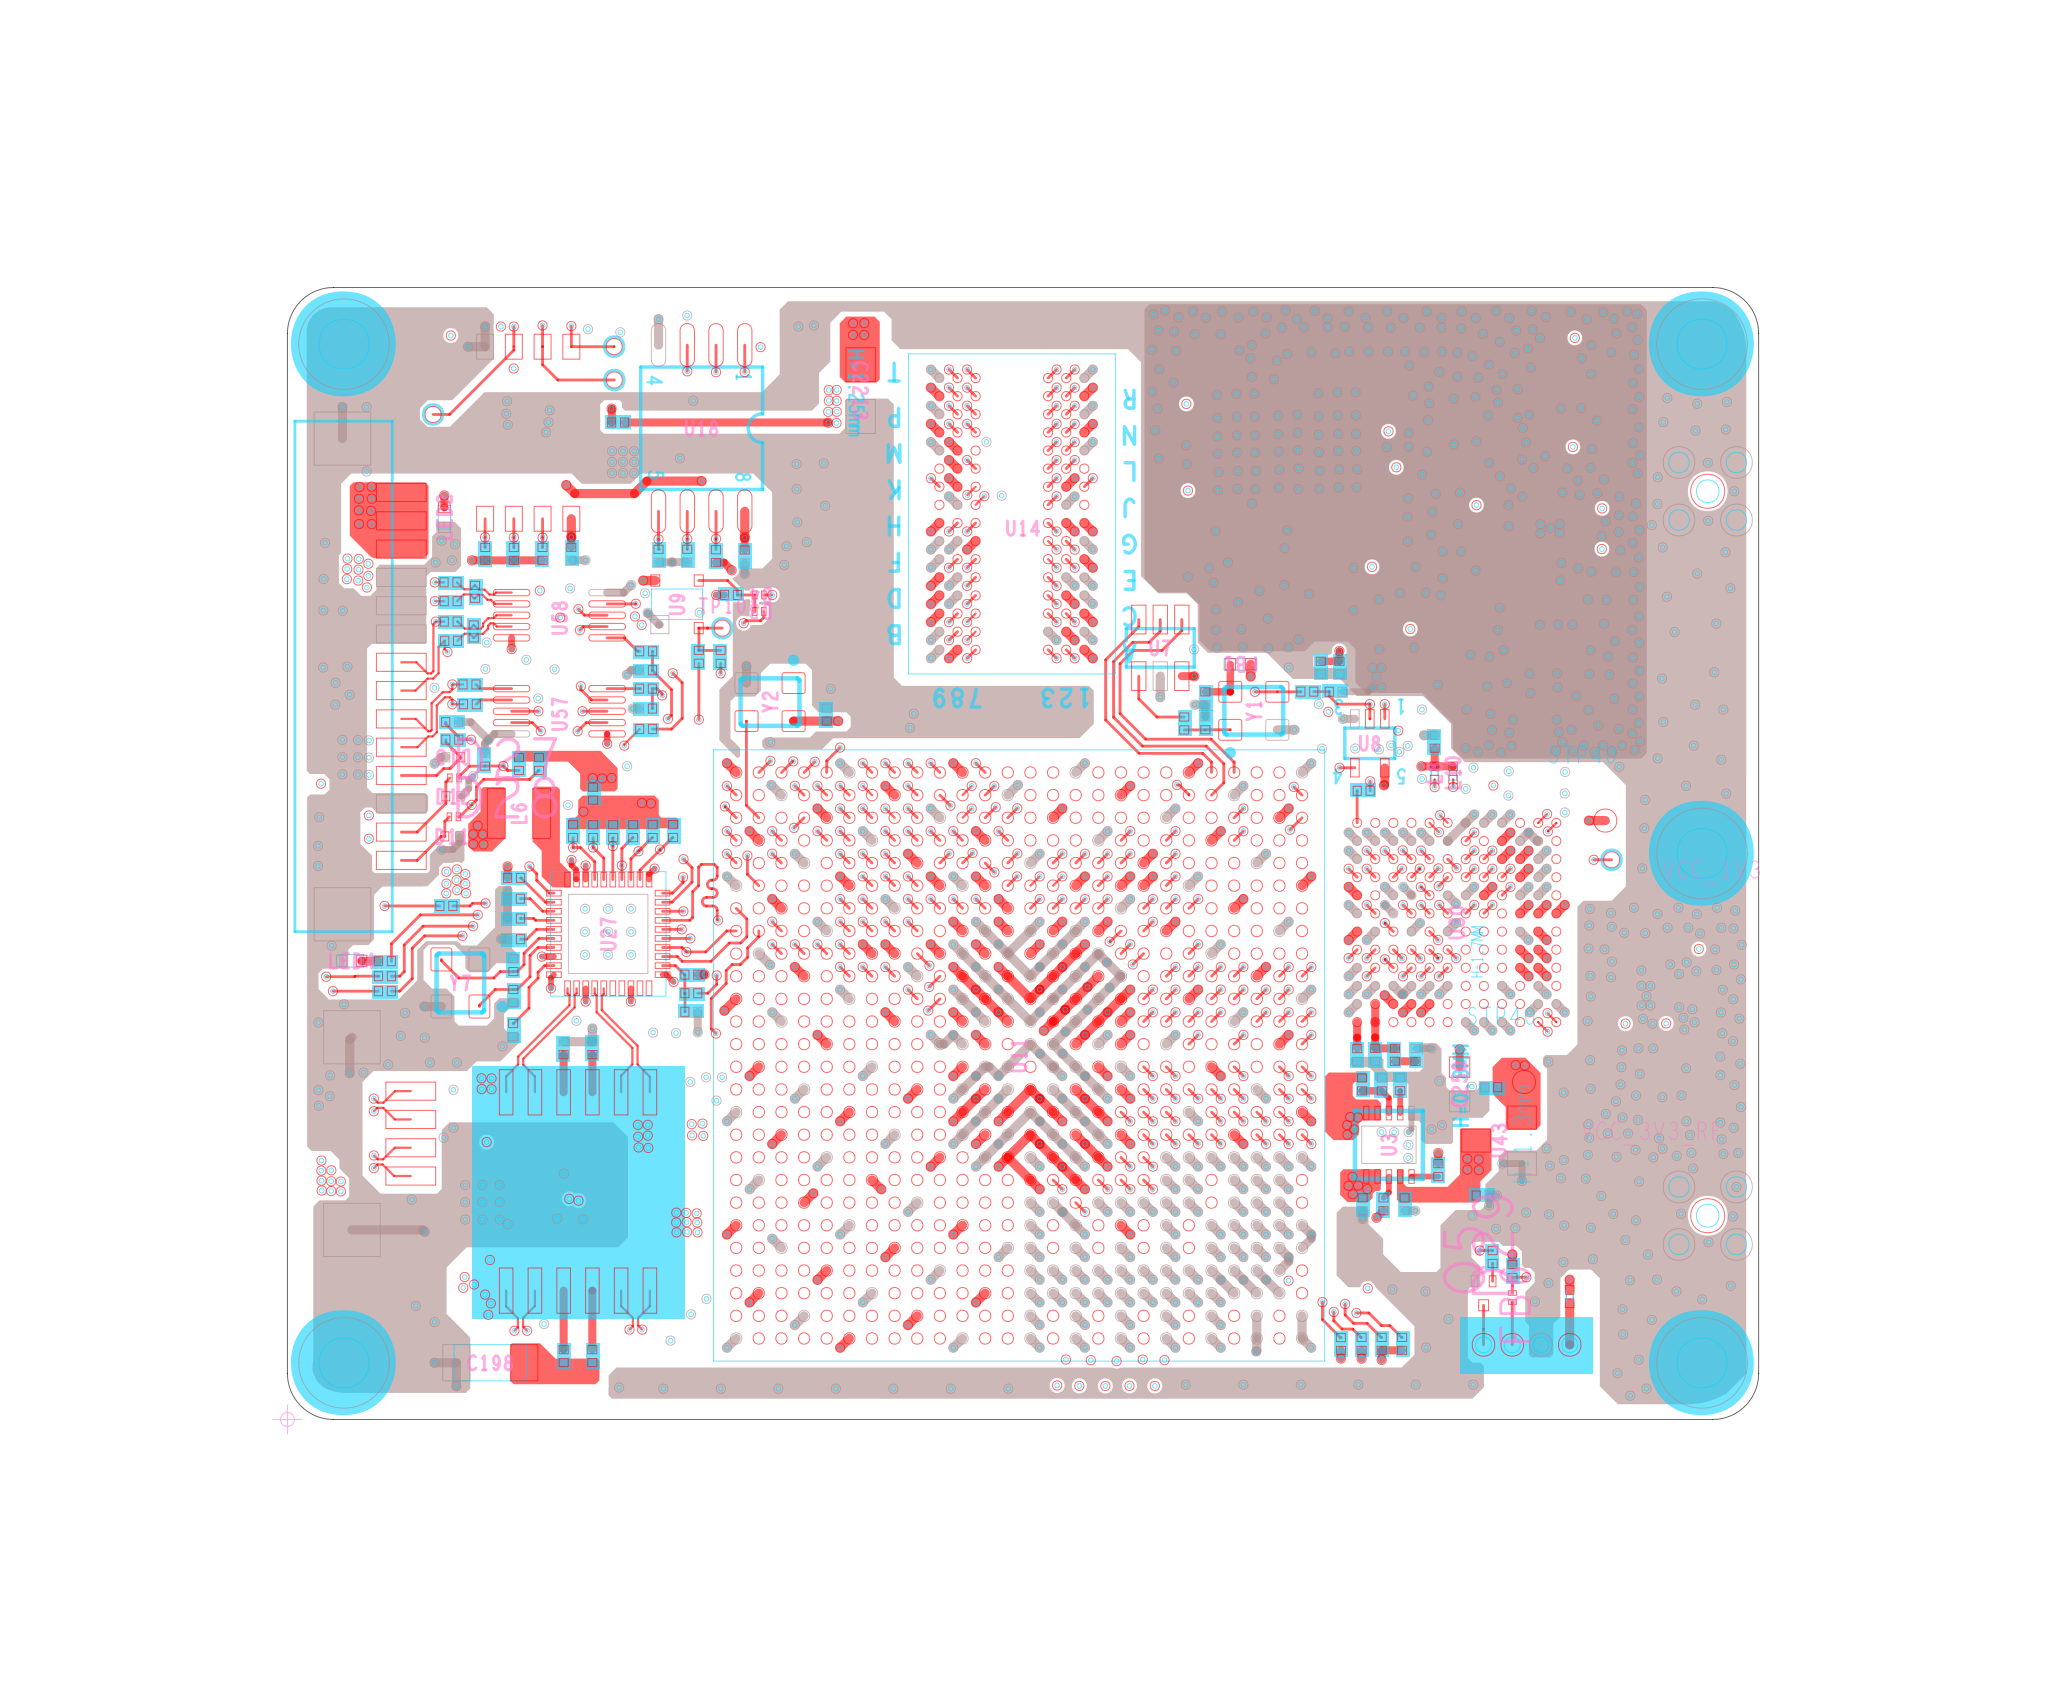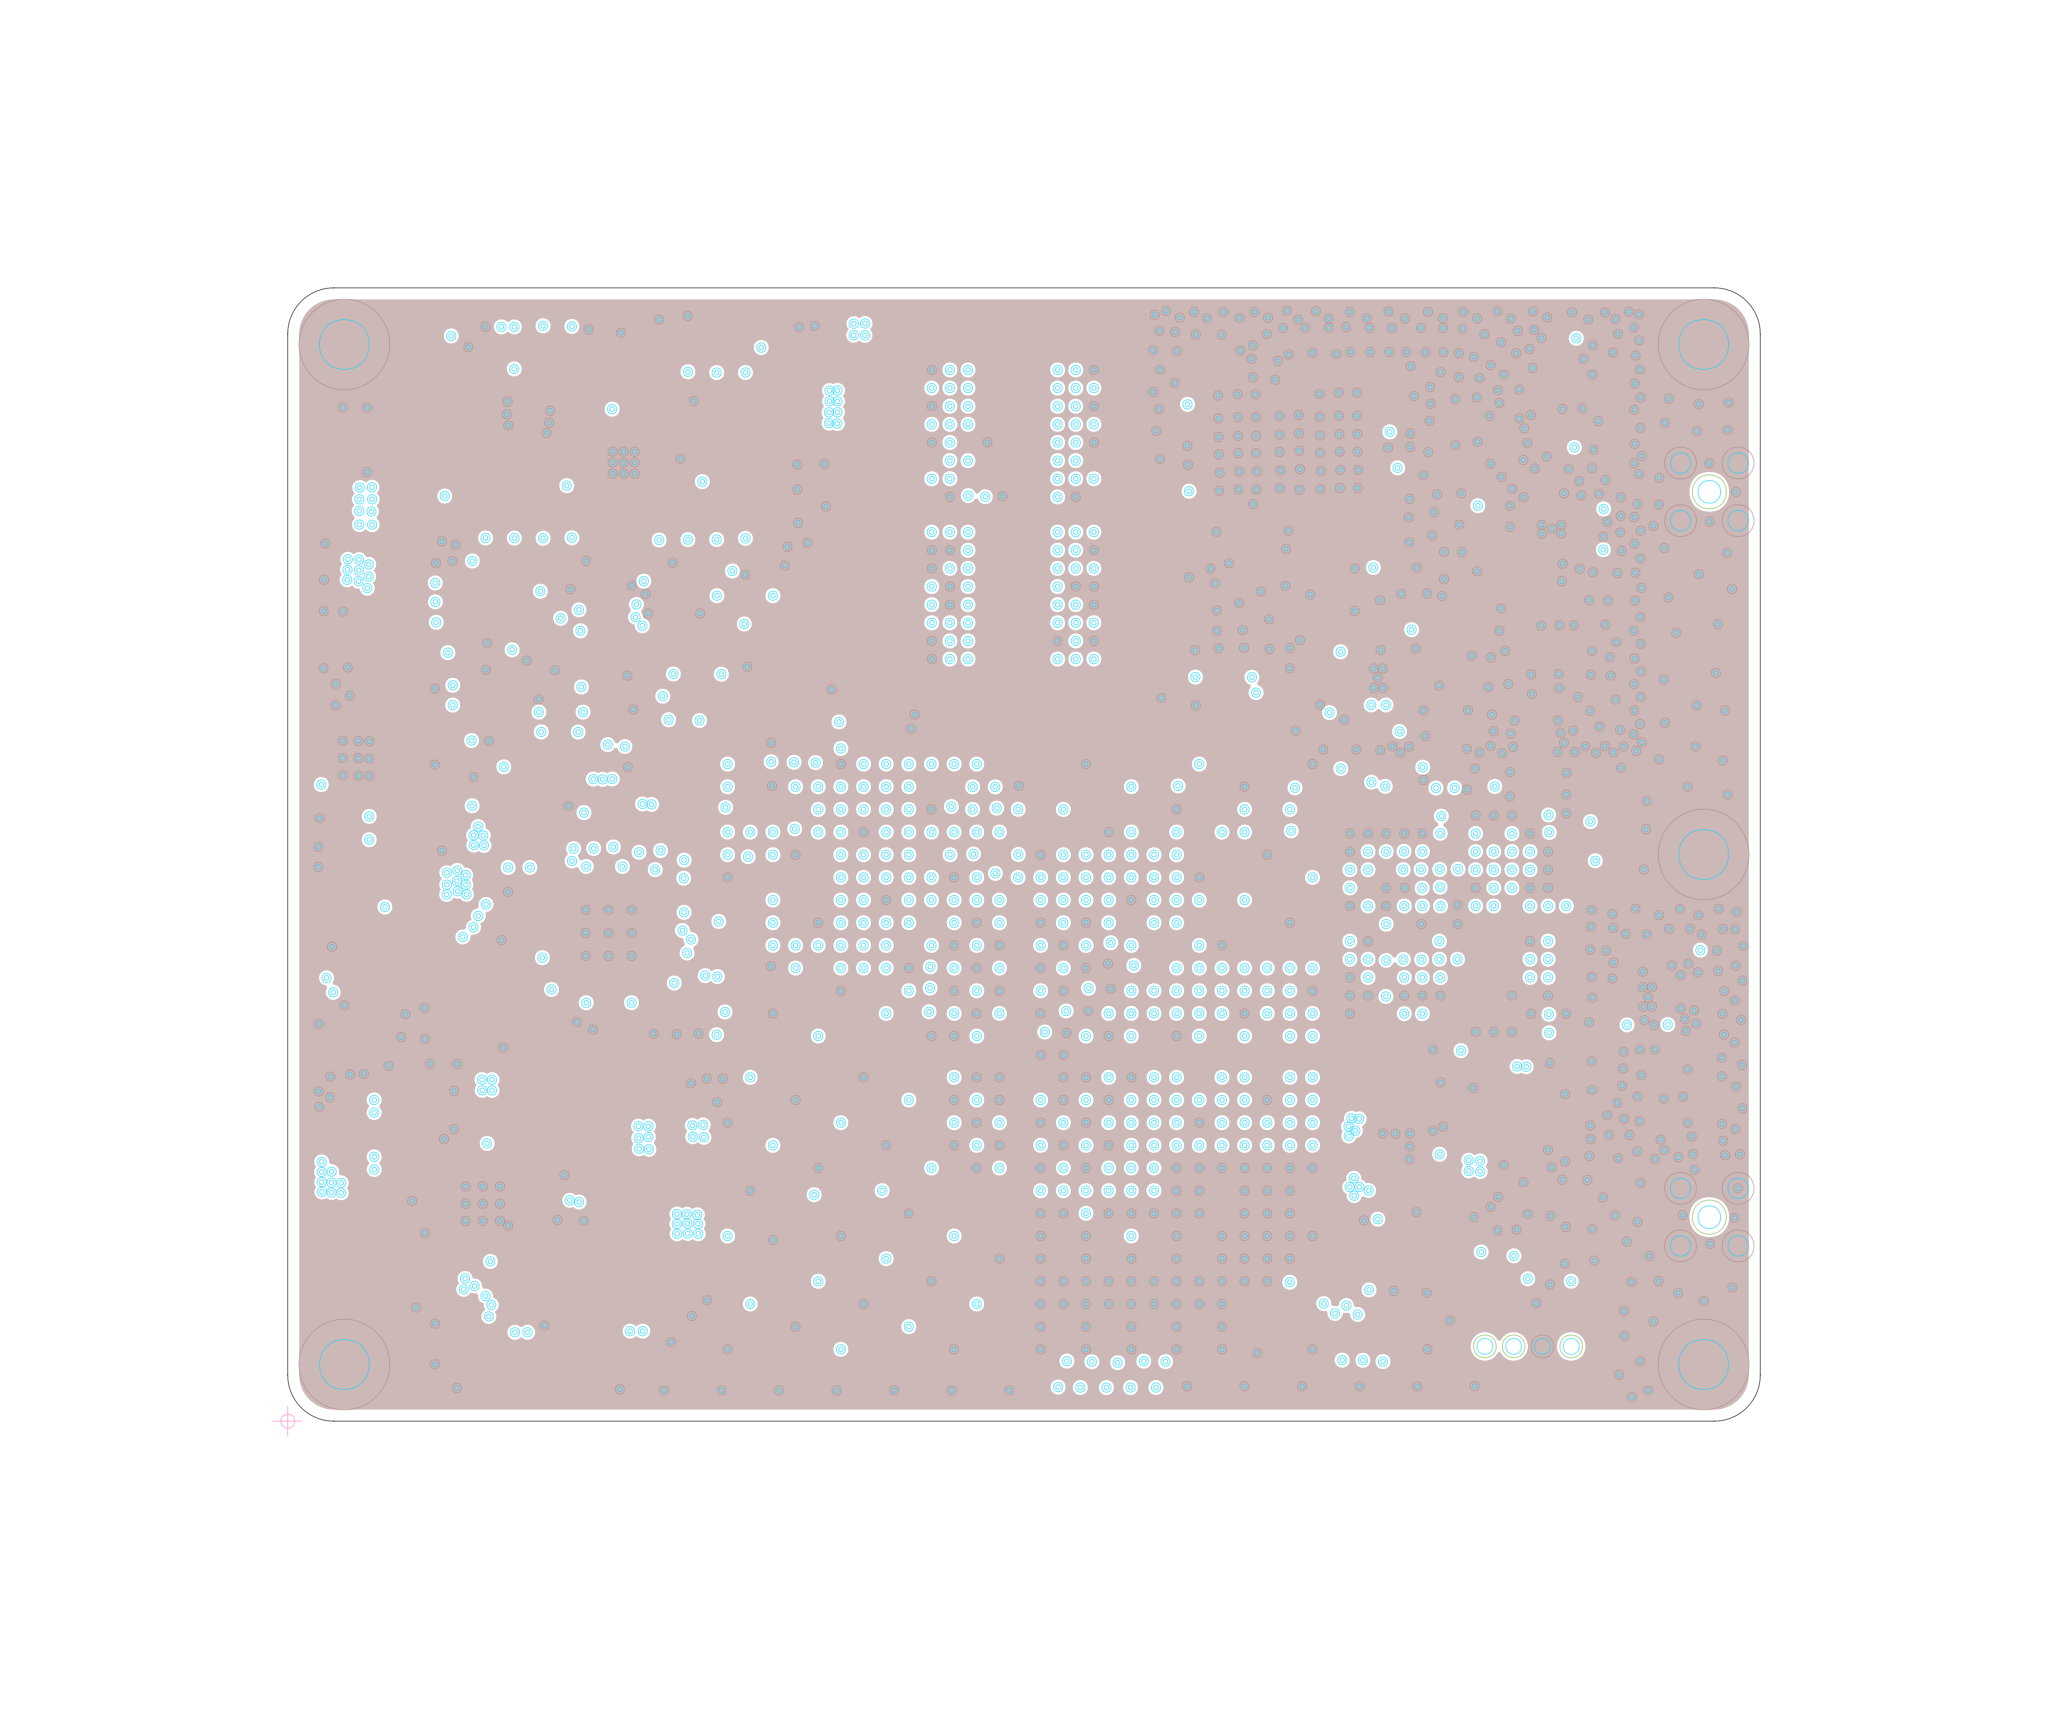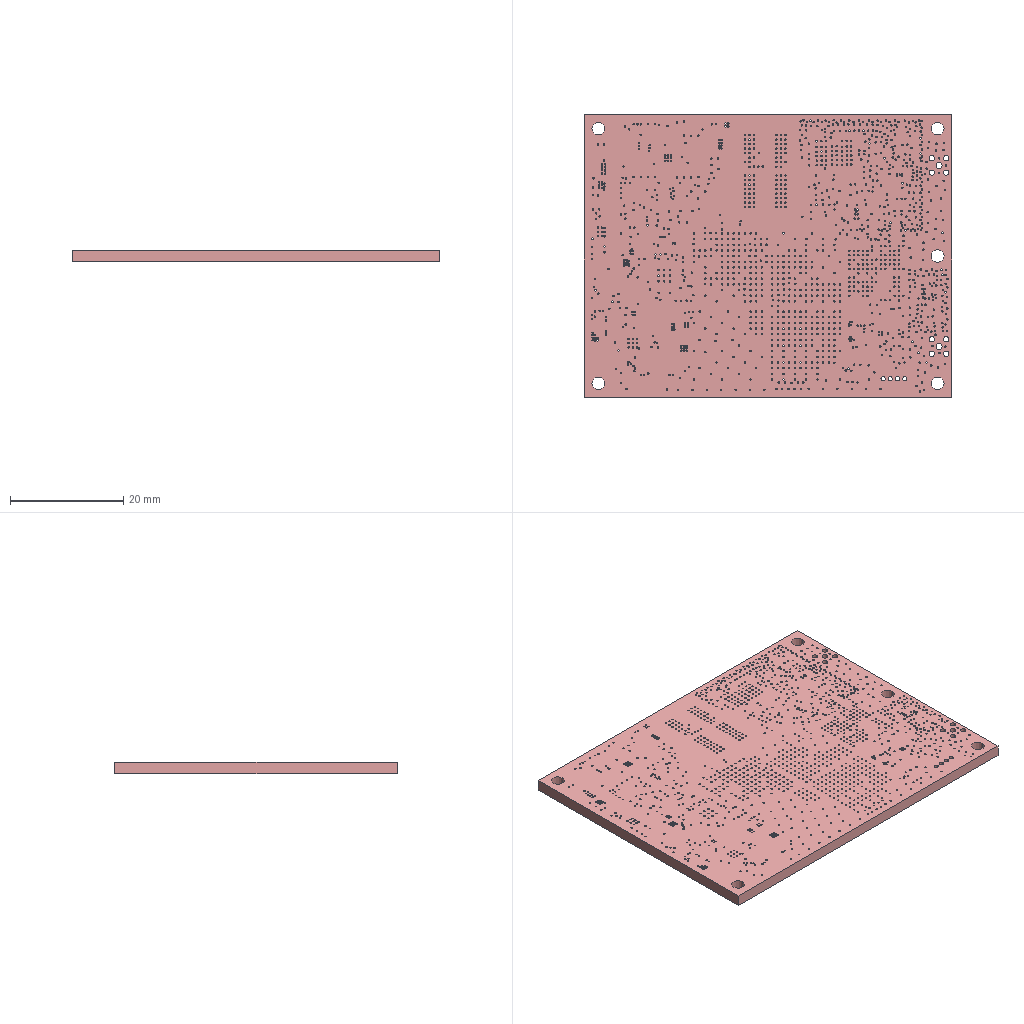Circuit board layout | Cadence Allegro | box 65 x 50 x 2.1 mm
Layer stack:
# Cadence Allegro layer stack of  (unit mm; from the constraint file cross-section; dielectric type: 0 not recorded (Allegro does not mark core vs prepreg), 3 surface material)
index,name,kind,layer,copper_thickness_mm,dielectric_type,dielectric_thickness_mm,dielectric_material,dielectric_constant
0,Top Surface,other,,,,,,
1,TOP,copper,TOP,0.0305,,,,
2,Dielectric1,dielectric,,,0,0.2032,FR-4,4.5
3,GND2,copper,GND2,0.0305,,,,
4,Dielectric2,dielectric,,,0,0.2032,FR-4,4.5
5,SIG3,copper,SIG3,0.0305,,,,
6,Dielectric3,dielectric,,,0,0.2032,FR-4,4.5
7,GND4,copper,GND4,0.0305,,,,
8,Dielectric4,dielectric,,,0,0.2032,FR-4,4.5
9,SIG5,copper,SIG5,0.0305,,,,
10,Dielectric5,dielectric,,,0,0.2032,FR-4,4.5
11,POWER6,copper,POWER6,0.0305,,,,
12,Dielectric6,dielectric,,,0,0.2032,FR-4,4.5
13,POWER7,copper,POWER7,0.0305,,,,
14,Dielectric7,dielectric,,,0,0.2032,FR-4,4.5
15,SIG8,copper,SIG8,0.0305,,,,
16,Dielectric8,dielectric,,,0,0.2032,FR-4,4.5
17,GND9,copper,GND9,0.0305,,,,
18,Dielectric9,dielectric,,,0,0.2032,FR-4,4.5
19,BOTTOM,copper,BOTTOM,0.0305,,,,
20,Bottom Surface,other,,,,,,
# drill layer pairs: low layer,high layer
drill_pair,TOP,BOTTOM
Part placement:
REFDES,COMP_VALUE,SYM_NAME,SYM_X,SYM_Y,SYM_ROTATE,SYM_MIRROR
19.2M1,LABTESTPOINT,LTPT28C49P,1682.500,1237.600,270.000,YES
BM2,PESD0402V05,TVS0402,2302.900,1808.200,270.000,YES
BM3,PESD0402V05,TVS0402,2449.720,655.643,0.000,YES
C5,10uF,C0603,286.024,197.343,0.000,YES
C6,0.1uF,C0201,724.022,543.299,270.000,YES
C7,22uF,C0805,665.661,542.059,270.000,YES
C8,10uF,C0603,318.824,537.637,0.000,YES
C9,0.1uF,C0201,54.812,516.432,270.000,YES
C10,22uF,C0805,108.678,493.106,270.000,YES
C13,10uF,C0603,416.339,197.441,180.000,YES
C14,0.1uF,C0201,728.827,237.131,90.000,YES
C15,22uF,C0805,666.330,227.719,90.000,YES
C16,1.8nF,C0201,1935.660,582.890,90.000,NO
C17,10uF,C0603,1883.012,461.320,180.000,YES
C18,0.1uF,C0201,87.615,1034.669,180.000,YES
C22,1.8nF,C0201,244.681,1180.295,180.000,YES
C23,22uF,C0805,128.811,1348.709,0.000,YES
C24,1.8nF,C0201,212.204,1022.668,270.000,YES
C25,0.1uF,C0201,1258.580,499.110,90.000,YES
C26,100uF,C1206,325.159,718.144,90.000,YES
C27,47pF,C0201,244.563,1120.874,0.000,YES
C28,5.6nF,C0201,255.879,1043.629,270.000,YES
C29,1nF,C0201,1596.644,1254.180,270.000,NO
C30,0.1uF,C0201,1548.378,1292.036,0.000,YES
C31,1nF,C0201,1548.400,1260.300,0.000,YES
C32,1nF,C0201,1823.407,912.707,90.000,YES
C33,0.1uF,C0201,1774.005,1265.716,180.000,NO
C34,0.1uF,C0201,1596.614,1210.662,270.000,NO
C35,0.1uF,C0201,640.123,1447.940,90.000,YES
C38,4.7uF,C0402_D,1775.174,1091.482,270.000,YES
C40,0.22uF,C0201,1077.257,841.159,180.000,YES
C41,47uF,C0805,1371.381,1101.177,0.000,YES
C42,4.7uF,C0402_D,1387.795,1040.736,180.000,YES
C43,0.1uF,C0201,1141.949,928.238,180.000,YES
C45,1nF,C0201,1242.366,1577.650,270.000,YES
C51,0.1uF,C0201,1307.305,1577.751,270.000,YES
C57,0.22uF,C0201,1217.977,682.823,270.000,YES
C63,4.7uF,C0402_D,1051.441,594.520,0.000,YES
C64,4.7uF,C0402_D,1589.632,854.746,180.000,YES
C72,0.1uF,C0201,1166.939,449.903,180.000,YES
C73,0.1uF,C0201,1456.305,879.956,180.000,YES
C76,100uF,C1206,974.311,323.013,90.000,YES
C77,100uF,C1206,865.433,323.013,90.000,YES
C78,22uF,C0805,1118.474,339.762,90.000,YES
C79,22uF,C0805,859.443,743.331,0.000,YES
C81,4.7uF,C0402_D,1272.709,557.816,0.000,YES
C82,4.7uF,C0402_D,1279.908,730.174,90.000,YES
C83,0.22uF,C0201,1410.508,728.216,0.000,YES
C84,0.22uF,C0201,1444.372,614.572,180.000,YES
C85,0.22uF,C0201,1293.406,661.163,90.000,YES
C86,0.22uF,C0201,1408.111,650.466,180.000,YES
C87,0.22uF,C0201,1412.348,766.906,180.000,YES
C88,0.22uF,C0201,1369.350,581.957,270.000,YES
C89,0.22uF,C0201,1410.275,540.199,270.000,YES
C90,0.22uF,C0201,1371.443,806.306,90.000,YES
C105,47uF,C0805,1247.390,358.875,90.000,YES
C111,4.7uF,C0402_D,1216.700,787.721,90.000,YES
C112,0.22uF,C0201,1178.454,843.967,0.000,YES
C128,0.1uF,C0201,1092.548,1747.161,270.000,YES
C129,0.1uF,C0201,1092.747,1811.327,270.000,YES
C130,0.1uF,C0201,1424.584,1809.463,270.000,YES
C148,2.2uf,C0201,493.774,1505.456,270.000,NO
C153,0.1uF,C0201,795.345,1500.843,270.000,NO
C192,22pF,C0201,392.953,736.512,270.000,NO
C193,22pF,C0201,393.051,790.154,90.000,NO
C196,10nF,C0201,530.547,645.781,90.000,NO
C197,10nF,C0201,480.315,645.718,90.000,NO
C198,1000pF/2KV,C1206L,352.902,98.630,180.000,NO
C200,4.7uF,C0402_D,599.841,925.082,90.000,YES
C201,1uF,C0201,562.484,931.646,90.000,YES
C202,0.1uF,C0201,525.830,931.423,90.000,YES
C203,4.7uF,C0402_D,384.332,1066.047,180.000,YES
C204,0.1uF,C0201,469.240,804.622,180.000,YES
C205,4.7uF,C0402_D,458.402,711.115,90.000,YES
C206,0.1uF,C0201,469.307,773.480,180.000,YES
C207,0.1uF,C0201,376.589,1017.151,180.000,YES
C208,0.1uF,C0201,495.724,933.417,90.000,YES
C209,0.1uF,C0201,702.545,708.974,0.000,NO
C210,4.7uF,C0402_D,639.311,811.579,0.000,YES
C211,0.1uF,C0201,646.118,773.311,0.000,YES
C212,0.1uF,C0201,518.756,755.736,270.000,YES
C213,0.1uF,C0201,646.181,927.531,90.000,YES
C214,0.1uF,C0201,597.400,756.185,270.000,YES
C235,10uF,C0603,1873.619,677.338,180.000,YES
C236,1uF,C0201,2221.902,1019.486,90.000,YES
C237,1nF,C0201,2221.552,968.852,270.000,YES
C238,1uF,C0201,2111.616,763.758,270.000,YES
C239,1nF,C0201,2187.502,861.766,180.000,YES
C240,10uF,C0603,2064.230,816.704,90.000,YES
C241,1uF,C0201,2216.812,755.996,270.000,YES
C242,1nF,C0201,2034.170,926.196,270.000,YES
C243,10uF,C0603,1813.246,806.873,270.000,YES
C244,1uF,C0201,1892.212,724.451,180.000,YES
C245,1nF,C0201,1909.173,760.533,180.000,YES
C246,1uF,C0201,2067.019,733.034,90.000,YES
C247,1nF,C0201,2029.903,732.936,90.000,YES
C248,1uF,C0201,2159.023,739.984,270.000,YES
C249,1nF,C0201,1866.964,855.399,0.000,YES
C250,10uF,C0603,2038.942,582.841,90.000,NO
C251,1uF,C0201,2216.180,805.108,90.000,YES
C252,1nF,C0201,2026.743,986.643,180.000,YES
C253,1uF,C0201,1897.867,1133.347,180.000,YES
C254,1nF,C0201,1790.172,912.677,270.000,YES
C255,1uF,C0201,1962.185,633.988,270.000,NO
C256,1nF,C0201,1892.085,634.125,90.000,NO
C257,1uF,C0201,2112.976,820.381,270.000,YES
C258,1nF,C0201,2144.295,865.365,270.000,YES
C259,100pF,C0201,1872.059,1093.328,0.000,NO
C260,3.9pF,C0201,2150.604,1106.815,270.000,YES
C261,10pF,C0201,1995.425,1124.121,270.000,YES
C264,1nF,C0201,1995.576,1178.612,90.000,NO
C265,10pF,C0201,2027.755,1124.250,270.000,YES
C266,3.9pF,C0201,2186.234,1106.815,270.000,YES
C277,3.9pF,C0201,1901.942,569.003,180.000,YES
C280,3.9pF,C0201,1902.563,534.354,180.000,YES
C290,0.1uF/50V,C0402_D,469.868,1686.807,270.000,YES
C292,47uF,C0805,909.681,1804.747,270.000,YES
C301,2.2uF,C0201,2093.993,577.906,180.000,NO
C302,1uF,C0201,2079.043,389.438,0.000,NO
C332,4.7uF,C0402_D,1924.200,1482.700,180.000,YES
C342,4.7uF,C0402_D,1932.900,1738.300,0.000,YES
C348,4.7uF,C0402_D,1566.387,1502.918,90.000,YES
C349,4.7uF,C0402_D,1563.400,1731.400,90.000,YES
C350,100pF,C0201,1917.471,1569.758,0.000,YES
C358,1nF,C0201,2098.000,1590.100,180.000,YES
C359,1uF,C0201,2097.938,1553.318,180.000,YES
C360,1nF,C0201,2144.600,1639.500,135.000,YES
C361,1nF,C0201,2186.300,1479.200,270.000,YES
C362,1nF,C0201,2211.600,1880.900,0.000,YES
C363,47pF,C0402_D,2243.800,1788.200,180.000,YES
C367,47pF,C0402_D,2187.800,1716.200,270.000,YES
C373,1nF,C0201,2436.758,829.343,270.000,YES
C374,1uF,C0201,2400.582,829.439,270.000,YES
C375,1nF,C0201,2469.658,700.462,270.000,YES
C376,1nF,C0201,2298.200,735.300,270.000,YES
C2117,10uF,C0603,1442.600,1368.600,270.000,YES
C2118,10uF,C0603,1088.826,1368.287,90.000,YES
C2119,0.1uF,C0201,1394.557,1603.340,90.000,YES
C2120,0.1uF,C0201,1423.604,1743.334,270.000,YES
C2134,4.7uF,C0402_D,820.527,1064.082,270.000,YES
C2136,0.1uF,C0201,1113.513,1677.586,315.000,YES
C2137,0.1uF,C0201,1426.740,1530.547,90.000,YES
C2147,47uF,C0805,1242.565,172.993,90.000,YES
C2148,0.1uF,C0201,938.091,1225.722,90.000,NO
C2149,0.1uF,C0201,1029.291,738.739,0.000,YES
C2156,0.22uF,C0201,862.396,801.165,0.000,YES
C2157,0.22uF,C0201,890.695,1062.591,0.000,YES
C2158,0.22uF,C0201,927.251,911.085,90.000,YES
C2159,0.22uF,C0201,802.992,1130.024,180.000,YES
C2160,0.22uF,C0201,1743.401,964.145,0.000,YES
C2161,0.22uF,C0201,1624.623,1122.244,180.000,YES
C2167,0.22uF,C0201,1113.954,983.796,180.000,YES
C2168,0.22uF,C0201,1158.269,1107.581,90.000,YES
C2169,0.22uF,C0201,1402.308,934.353,90.000,YES
C2170,0.22uF,C0201,1028.758,1119.040,0.000,YES
C2171,0.22uF,C0201,1089.198,1466.037,270.000,YES
C2172,0.22uF,C0201,1434.733,1468.010,90.000,YES
C2173,0.22uF,C0201,1096.456,1527.792,90.000,YES
C2195,0.22uF,C0201,1764.658,507.329,90.000,YES
C2196,0.22uF,C0201,1373.689,882.035,180.000,YES
C2197,0.22uF,C0201,1445.529,463.203,0.000,YES
C2198,0.22uF,C0201,1703.507,678.991,0.000,YES
C2199,0.22uF,C0201,1724.008,827.593,270.000,YES
C2200,0.22uF,C0201,1677.404,459.359,90.000,YES
C2208,10uF/50V,C0805,417.528,1706.050,270.000,YES
C2209,10uF/50V,C0805,345.033,1705.964,270.000,YES
C2211,0.1uF,C0201,692.712,1608.576,270.000,YES
C2213,47uF,C0805,997.100,1789.300,270.000,NO
C2217,4.7uF,C0402_D,128.217,1280.465,0.000,YES
C2218,82pF,C0201,623.955,1834.251,90.000,YES
C2219,0.1uF,C0201,457.970,1242.692,270.000,YES
C2220,0.1uF,C0201,469.287,1197.143,180.000,YES
C2222,0.1uF,C0201,556.158,1147.219,90.000,YES
C2224,0.1uF,C0201,415.618,1347.696,90.000,YES
C2229,4.7uF/35V,C0603,201.274,1689.628,0.000,YES
C2277,47pF,C0201,2186.663,1282.807,270.000,YES
C2279,47pF,C0201,2071.400,534.200,180.000,YES
C2280,100pF,C0201,1603.358,1509.253,270.000,YES
C2281,100pF,C0201,1552.400,1784.200,180.000,YES
C2282,100pF,C0201,1926.400,1780.400,0.000,YES
C2283,2.2nF,C0201,1708.700,1529.200,0.000,YES
C2291,100pF,C0201,1917.700,1526.700,0.000,YES
C2315,0.22uF,C0201,1212.305,1012.039,90.000,YES
C2321,0.22uF,C0201,1587.467,1044.722,0.000,YES
C2323,1uF,C0201,468.831,374.204,90.000,YES
C2327,1uF,C0201,1870.267,374.202,270.000,NO
C2328,1uF,C0201,1943.152,374.135,270.000,NO
C2329,220pF,C0201,150.237,392.788,180.000,YES
C2330,220pF,C0201,545.840,358.676,0.000,YES
C2331,220pF,C0201,545.092,405.027,0.000,YES
C2332,0.1uF,C0201,684.239,1359.245,180.000,YES
C2333,47nF,C0201,478.700,1802.900,0.000,YES
C2334,4.7uF,C0402_D,700.200,1706.400,90.000,YES
C2335,10uF/50V,C0805,222.600,1760.100,0.000,YES
C2336,1nF,C0201,1797.358,1307.352,270.000,NO
C2337,0.1uF,C0201,1829.958,1307.223,270.000,NO
C2338,0.1uF,C0201,1899.318,1363.463,90.000,YES
C2339,1nF,C0201,1780.900,1311.300,270.000,YES
C2340,1nF,C0201,1972.100,1299.700,0.000,YES
C2341,1nF,C0201,1983.500,1311.100,270.000,YES
C2342,1nF,C0201,1791.900,1322.900,0.000,YES
D3,TPMEG4002ESFYL,D0201,820.750,1405.124,180.000,NO
D4,TPMEG4002ESFYL,D0201,820.750,1433.838,180.000,NO
D11,PESD0201V05,TVS0201,286.730,1014.006,0.000,NO
D12,PESD0201V05,TVS0201,288.509,1083.782,0.000,NO
D13,PESD0201V05,TVS0201,288.509,1151.657,180.000,NO
D14,PESD0201V05,TVS0201,316.658,1243.260,180.000,YES
D15,PESD0201V05,TVS0201,315.658,1278.460,180.000,YES
D16,PESD0201V05,TVS0201,291.288,1351.156,180.000,YES
D17,PESD0201V05,TVS0201,290.788,1386.556,180.000,YES
D18,PESD0201V05,TVS0201,188.454,431.494,180.000,YES
D19,PESD0201V05,TVS0201,188.454,465.494,180.000,YES
D20,PESD0201V05,TVS0201,188.454,530.382,180.000,YES
D21,PESD0201V05,TVS0201,188.454,564.382,180.000,YES
D25,SMF28CA-MS,SOD-123FL,91.657,1664.360,270.000,YES
D27,TPMEG4002ESFYL,D0201,290.463,1115.710,0.000,NO
D28,TPMEG4002ESFYL,D0201,289.483,1048.010,0.000,NO
D29,TPMEG4002ESFYL,D0201,2130.790,212.103,90.000,NO
F1,06H1500D,R0603,197.697,1594.500,270.000,YES
FB1,BLM15PD121SN1,L0402_D,1657.809,1313.172,0.000,NO
FB2,BLM15PD121SN1,L0402_D,1620.700,1292.100,180.000,YES
FB3,BLM15PD121SN1,L0402_D,1157.476,628.844,0.000,YES
FB4,BLM03PX121SN1D,L0201,1273.260,865.644,90.000,YES
FB6,BLM03PX121SN1D,L0201,2230.400,213.700,90.000,NO
FB10,BLM15PD121SN1,L0402_D,2205.025,1840.093,180.000,YES
J4,B2S_4PIN,DIP1X4_1_27,2155.500,129.800,0.000,NO
J23,MMCX,DL-MMCX-KWE-90,2470.500,1614.173,90.000,NO
J26,MMCX,DL-MMCX-KWE-90,2470.500,354.331,90.000,NO
J28,HEADER 12X2,1MM25_14PIN,146.857,1292.147,270.000,NO
J31,HEADER 4,H-1MM25_4PIN,163.327,497.157,270.000,NO
J33,AFC01-S08FCA-00,AFC01-S08FCA-00,1829.898,228.583,180.000,YES
L1,FTC252012S1R5MBCA,1008,540.195,521.618,270.000,YES
L2,FTC252012S1R5MBCA,1008,148.310,275.551,90.000,YES
L3,FTC252012S1R5MBCA,1008,550.063,246.900,270.000,YES
L4,FXL0420-1R0-M,SMD_0420,170.330,882.297,270.000,YES
L6,SWPA3015S2R2MT,1008,402.739,1053.869,90.000,NO
L7,5.1nH/DNP,L0201,2011.402,1169.406,180.000,YES
L8,27nH,L0201,1995.420,1124.349,90.000,NO
L9,3.9nH,L0201,2168.911,1152.327,180.000,YES
L10,27nH,L0201,2027.555,1124.403,90.000,NO
L18,3.9nH,L0201,1948.531,551.972,90.000,YES
L23,FTC303020D3R3MBCA,SMD_30X30,798.598,1692.557,270.000,YES
L32,MLG0603P2N7CT000,L0201,2185.996,1619.864,90.000,YES
L34,MLG0603P2N7CT000,L0402_D,2451.900,746.500,0.000,YES
L48,SLQW1005C47NJT,L0402_D,2345.321,818.011,180.000,YES
L50,SLQW1005C47NJT,L0402_D,2104.492,1513.489,0.000,YES
L51,SCW1005C43NJST,L0201,1827.700,1311.400,90.000,YES
LED2,GREEN,D0402,272.922,1568.962,270.000,NO
LED4,GREEN,D0402,111.720,797.524,180.000,NO
LED5,GREEN,D0402,51.842,846.034,90.000,YES
LED6,GREEN,D0402,51.940,728.238,90.000,YES
LED7,GREEN,D0402,51.744,611.422,90.000,YES
Q5,MMBT3904M,SOT-723,2080.600,219.500,90.000,NO
Q6,SMP1330-005LF,SOT-23,2069.000,1700.400,270.000,YES
Q7,SMP1330-005LF,SOT-23,2429.775,560.884,270.000,YES
R3,4.7K,R0201,286.470,1212.701,0.000,NO
R5,4.7K,R0201,272.876,1635.896,90.000,YES
R8,1K,R0201,286.729,1182.161,180.000,NO
R11,49.9K,R0201,545.130,437.245,0.000,YES
R12,100K,R0201,150.292,359.777,0.000,YES
R14,33K,R0201,351.870,252.657,90.000,YES
R15,26.7K,R0201,192.143,366.255,90.000,YES
R16,39.2K,R0201,498.982,416.185,90.000,YES
R17,10K,R0201,2001.847,433.666,90.000,NO
R18,100K,R0201,545.848,325.759,0.000,YES
R19,6.25K,R0201,1869.212,582.663,270.000,NO
R21,49.9K,R0201,501.157,336.883,90.000,YES
R22,10K,R0201,1903.567,582.662,90.000,NO
R23,52.3K,R0201,58.665,1269.272,270.000,YES
R26,22.1K,R0201,244.693,1213.000,180.000,YES
R27,100K,R0201,157.169,1036.713,0.000,YES
R29,4.7K,R0201,244.465,1085.882,180.000,YES
R30,33K,R0201,244.591,1244.882,0.000,YES
R31,12.1K,R0201,1882.868,1206.915,270.000,YES
R32,1K,R0201,1908.000,1206.900,90.000,YES
R33,1K,R0201,1559.872,1210.367,270.000,NO
R34,10K,R0201,1823.490,1265.486,0.000,NO
R35,22R,R0201,715.618,1326.303,90.000,NO
R36,10K,R0201,788.203,1001.491,180.000,YES
R39,10K,R0201,645.471,1501.994,270.000,NO
R40,10K,R0201,745.600,1853.416,270.000,YES
R41,10K,R0201,912.094,992.624,90.000,YES
R42,10K,R0201,343.643,1147.358,90.000,NO
R43,1K,R0201,1021.029,809.743,180.000,YES
R44,1K,R0201,1077.222,808.816,180.000,YES
R45,80R6,R0201,1485.360,963.993,45.000,YES
R46,80R6,R0201,1485.489,924.722,225.000,YES
R47,1K,R0201,1228.228,1523.953,270.000,YES
R48,1K,R0201,1274.399,1577.752,270.000,YES
R65,10K,R0201,695.386,1502.143,270.000,NO
R68,10K,R0201,695.291,1853.269,270.000,YES
R72,10K,R0201,745.291,1501.340,270.000,NO
R74,1K,R0201,1397.518,69.604,90.000,YES
R76,1K,R0201,169.635,797.019,180.000,NO
R77,1K,R0201,276.454,893.059,180.000,NO
R80,1K,R0201,169.537,770.853,180.000,NO
R83,1K,R0201,169.480,744.834,180.000,NO
R115,240R,R0201,1184.539,1691.754,180.000,YES
R117,4.7K,R0201,1389.417,1848.701,180.000,YES
R118,80R6,R0201,1328.419,960.099,180.000,YES
R123,10K,R0201,393.877,1505.189,90.000,NO
R125,10K,R0201,344.091,1505.292,90.000,NO
R126,10K,R0201,443.731,1505.267,90.000,NO
R130,10K/DNP,R0201,795.502,1853.595,90.000,YES
R184,75R,R0201,480.586,110.232,270.000,NO
R185,75R,R0201,530.290,110.164,270.000,NO
R187,4.7K,R0201,394.268,835.260,180.000,NO
R188,4.7K,R0201,394.205,941.760,180.000,NO
R189,4.7K,R0201,394.075,871.189,180.000,NO
R190,2.49K,R0201,392.555,677.350,270.000,NO
R191,4.7K,R0201,431.984,985.586,0.000,YES
R192,4.7K,R0201,394.004,905.638,180.000,NO
R195,4.7K,R0201,670.783,1023.252,270.000,NO
R196,4.7K,R0201,496.854,1023.142,90.000,NO
R197,4.7K,R0201,531.697,1023.083,90.000,NO
R200,4.7K,R0201,566.650,1023.071,90.000,NO
R202,4.7K,R0201,601.295,1023.071,90.000,NO
R204,0R,R0201,531.598,1088.233,270.000,NO
R206,4.7K,R0201,635.232,1023.157,270.000,NO
R208,4.7K,R0201,702.546,773.497,180.000,NO
R209,1K,R0201,702.400,773.866,0.000,YES
R210,0R,R0201,702.561,741.253,180.000,NO
R245,10K,R0201,2079.833,1091.217,270.000,YES
R246,10K,R0201,2127.339,904.440,180.000,YES
R247,0R,R0201,2221.957,923.169,270.000,YES
R248,1R,R0201,1926.433,634.126,90.000,NO
R249,1R,R0201,2112.818,865.462,90.000,YES
R250,0R,R0201,1860.783,633.732,90.000,NO
R251,14.3k,R0201,2111.500,1031.000,270.000,YES
R252,110K,R0201,634.922,1794.486,180.000,YES
R253,100K,R0201,444.197,1826.286,180.000,YES
R254,15K,R0201,590.857,1834.022,270.000,YES
R262,0R,R0201,1917.600,1635.300,180.000,YES
R272,10K,R0201,493.733,1866.579,270.000,YES
R2100,10K,R0201,443.730,1866.483,270.000,YES
R2104,22R,R0201,753.587,1326.130,90.000,NO
R2119,0R,R0805,990.095,1796.746,90.000,YES
R2120,22.1K,R0201,522.877,1836.923,270.000,YES
R2122,10K,R0201,575.200,1733.800,0.000,NO
R2123,1K,R0201,654.514,1834.138,90.000,YES
R2125,10K,R0201,494.484,1242.976,90.000,YES
R2137,10K,R0201,478.841,1372.820,180.000,YES
R2138,10K,R0201,478.573,1419.349,0.000,YES
R2143,0R,R0201,289.409,1314.547,0.000,YES
R2144,0R,R0201,623.849,1200.644,180.000,NO
R2145,0R,R0201,317.323,1243.799,180.000,NO
R2147,0R,R0201,316.732,1278.248,180.000,NO
R2169,22R,R0201,2236.000,1722.500,270.000,YES
R2173,10K,R0201,2386.838,667.842,180.000,YES
R2174,10K,R0201,2338.657,667.942,180.000,YES
R2177,10K,R0201,2265.058,1573.176,270.000,YES
R2179,10K,R0201,2265.158,1524.895,270.000,YES
R2188,10K,R0201,1917.600,1602.000,180.000,YES
R2190,0R,R0201,284.687,1354.146,180.000,NO
R2191,0R,R0201,283.931,1423.018,180.000,NO
R2192,0R,R0201,283.665,1455.865,180.000,NO
R2193,0R,R0201,284.052,1387.546,180.000,NO
R2194,4.7K,R0201,1442.216,69.487,90.000,YES
R2195,4.7K,R0201,1354.283,70.373,90.000,YES
R2196,510R,R0201,1527.793,69.626,90.000,YES
R2197,4.7K,R0201,1868.438,131.396,270.000,NO
R2198,4.7K,R0201,1832.513,131.184,270.000,NO
R2199,4.7K,R0201,1903.379,131.467,270.000,NO
R2200,4.7K,R0201,1938.910,131.451,270.000,NO
R2201,1K,R0201,1509.015,634.524,180.000,YES
R2202,0R,R0201,1485.476,69.694,90.000,YES
R2203,10K,R0201,1906.538,374.210,90.000,NO
R2205,22R,R0201,382.511,1878.357,180.000,YES
R2206,1K,R0201,623.851,1335.915,180.000,NO
R2207,4.7K,R0201,623.737,1303.045,180.000,NO
R2208,1K,R0201,623.573,1270.951,180.000,NO
R2209,4.7K,R0201,623.727,1236.279,180.000,NO
R2210,10K,R0201,324.079,1370.447,270.000,NO
R2211,10K,R0201,326.235,1439.226,270.000,NO
R2216,4.7K,R0201,771.456,1433.838,0.000,NO
R2217,10K,R0201,402.676,1139.861,270.000,NO
R2218,10K,R0201,437.576,1139.842,270.000,NO
R2219,10K,R0201,2130.800,258.100,270.000,NO
R2220,10K,R0201,2096.400,282.500,90.000,NO
R2221,110K,R0201,478.500,1769.400,0.000,YES
R2222,732K,R0201,680.600,1771.600,0.000,YES
R2223,15K,R0201,594.400,1786.600,270.000,YES
R2224,0R,R0201,1834.200,1526.700,180.000,YES
R2225,0R,R0201,1644.600,1520.300,0.000,YES
R2226,0R,R0201,1915.200,1821.200,270.000,YES
R2227,0R,R0201,1563.800,1821.200,270.000,YES
R2228,15K,R0201,1930.942,1363.080,90.000,YES
R2229,15K,R0201,1814.939,1268.642,180.000,YES
SCR5,SCR,HOLE2_2_4,98.425,98.425,0.000,NO
SCR6,SCR,HOLE2_2_4,98.425,1870.079,0.000,NO
SCR7,SCR,HOLE2_2_4,2460.630,1870.079,0.000,NO
SCR8,SCR,HOLE2_2_4,2460.630,98.425,0.000,NO
SCR9,SCR,HOLE2_2_4,2460.630,984.252,0.000,NO
TP3,LABTESTPOINT,LTPT28C49P,568.302,1865.724,0.000,NO
TP4,LABTESTPOINT,LTPT28C49P,568.596,1807.708,0.000,NO
TP5,LABTESTPOINT,LTPT28C49P,253.330,1747.732,0.000,NO
TP6,LABTESTPOINT,LTPT28C49P,443.254,1470.882,0.000,YES
TP7,LABTESTPOINT,LTPT28C49P,393.176,1491.070,0.000,YES
TP8,LABTESTPOINT,LTPT28C49P,344.078,1459.808,0.000,YES
TP9,LABTESTPOINT,LTPT28C49P,1673.500,1475.500,90.000,YES
TP10,LABTESTPOINT,LTPT28C49P,756.280,1376.208,0.000,NO
TP11,LABTESTPOINT,LTPT28C49P,2303.300,973.300,0.000,NO
U2,EA3059C,QFN_24,342.343,375.673,0.000,YES
U3,TPS74801DRCR,TPS74901DRCR,1915.952,477.667,90.000,NO
U6,TPS54821,PVQFN14,126.252,1150.697,180.000,YES
U7,DAC121S101,SOT-23-6,1518.249,1341.888,0.000,NO
U8,74LVC1G126GW,SC-70,1882.756,1175.859,180.000,NO
U9,MAX811R,SOT-143,677.659,1417.629,270.000,NO
U11,XC7Z035-2FFG676I,FPGA_ZYNQ7045_676,1272.709,633.016,90.000,NO
U14,MT41K256M16TW-107,FBGA_DDR4_96P,1260.086,1574.783,180.000,NO
U17,MKDV32GCL-STP,MKDV32GCL-STP,418.803,1715.984,180.000,NO
U18,W25Q256JVEIQ,SO8-25X75-200,720.472,1723.827,180.000,NO
U27,RTL8211F-CG,QFN40_5R00X5R00X0R90_T,558.071,844.390,90.000,NO
U30,AD9363,CSPBGA-144-0_8-AD9361,2033.893,864.252,90.000,NO
U31,HHM17147A1,B1608-LDB18,2011.544,1234.650,90.000,YES
U32,HHM17147A1,B1608-LDB18,2169.080,1216.783,90.000,YES
U36,HHM17147A1,B1608-LDB18,2008.188,551.903,0.000,YES
U39,SY8308,SY8308RBC,583.491,1664.341,270.000,YES
U43,RT9166-33GVL,SOT-23,2107.534,485.077,90.000,NO
U44,ZD9098,DFN2X2-8P,2196.100,1549.000,90.000,YES
U46,LX8625EH,DFN6_1_1_0_7MM,2179.600,1788.100,0.000,YES
U49,ZD9098,DFN2X2-8P,2362.800,736.700,0.000,YES
U56,HC_027,HC_027,505.437,396.535,180.000,NO
U57,MAX3311,MSOP-10_1,472.949,1231.571,90.000,NO
U58,ISL3156EIUZ-T,MSOP-10_1,473.043,1398.583,90.000,NO
U61,GCM1437A,PA-14-1_06-GCM1437A,1739.300,1701.100,270.000,YES
U65,TA2485A,TA2494A,2186.200,1381.900,90.000,YES
U66,TA2485A,TA2494A,2168.500,534.200,0.000,YES
U1290,SN74AVC4T245RSVR,UQFN-16,593.620,1305.631,180.000,YES
U1291,TA2485A,TA2494A,1780.900,1436.800,270.000,YES
U1292,ZD9019,DFN2X2-8P,1895.300,1290.200,0.000,YES
VCC_1V0,T POINT F,STP40,408.800,779.300,0.000,YES
VCC_1V3,T POINT F,STP40,2292.395,1041.498,0.000,NO
VCC_1V8,T POINT F,STP40,753.600,297.100,0.000,YES
VCC_1V35,T POINT F,STP40,617.005,422.698,0.000,YES
VCC_3V3_RF,T POINT F,STP40,2150.895,586.998,0.000,NO
VCC_3V3,T POINT F,STP40,73.505,368.798,0.000,YES
VCC_5V,T POINT F,LTPT28C49P,839.100,1812.900,0.000,YES
VCC_IN,T POINT F,STP40,336.303,1591.907,0.000,YES
Y1,DSA321 19.2MHZ,OSC2520,1680.915,1232.392,90.000,NO
Y2,33MHz,OSC2520,839.451,1247.514,270.000,NO
Y7,25MHz,OSC2520,300.827,759.126,180.000,NO
Pad and via stacks, first 108 of 181 lines:
# Allegro (Cadence) via spans and padstacks; design units: ("mils" 3 1000)
# via spans: padstack,start_layer,end_layer,net_example,count
VIA8-16,ETCH/TOP,ETCH/BOTTOM,PLAN0_B-,1562
# Allegro padstack definitions: name,start_layer,end_layer,drill,plating,holeType,type
TPT28C49P,"ETCH/TOP","ETCH/TOP",0.0,"NON_PLATED","none","smd"
SMD25_20,"ETCH/TOP","ETCH/TOP",0.0,"PLATED","none","smd"
R0_455X0_5,"ETCH/TOP","ETCH/TOP",0.0,"NON_PLATED","none","smd"
R1_5X1_3,"ETCH/TOP","ETCH/TOP",0.0,"NON_PLATED","none","smd"
SMD22_20-A,"ETCH/TOP","ETCH/TOP",0.0,"PLATED","none","smd"
R1_4X2_6,"ETCH/TOP","ETCH/TOP",0.0,"PLATED","none","smd"
R0_9X0_9,"ETCH/TOP","ETCH/TOP",0.0,"PLATED","none","smd"
R0_7X0_5,"ETCH/TOP","ETCH/TOP",0.0,"PLATED","none","smd"
SMD1R20X1R60,"ETCH/TOP","ETCH/TOP",0.0,"PLATED","none","smd"
SMD3R00X1R50,"ETCH/TOP","ETCH/TOP",0.0,"NON_PLATED","none","smd"
SMD100_180,"ETCH/TOP","ETCH/TOP",0.0,"PLATED","none","smd"
R032X024S,"ETCH/TOP","ETCH/TOP",0.0,"PLATED","none","smd"
SMD25_40,"ETCH/TOP","ETCH/TOP",0.0,"PLATED","none","smd"
SMD52_52,"ETCH/TOP","ETCH/TOP",0.0,"PLATED","none","smd"
BALL40,"ETCH/TOP","ETCH/TOP",0.0,"PLATED","none","smd"
R1_65X1_6,"ETCH/TOP","ETCH/TOP",0.0,"PLATED","none","smd"
R1_0X1_5,"ETCH/TOP","ETCH/TOP",0.0,"PLATED","none","smd"
REC87X31,"ETCH/TOP","ETCH/TOP",0.0,"PLATED","none","smd"
SMD67_224,"ETCH/TOP","ETCH/TOP",0.0,"PLATED","none","smd"
SMD165_165,"ETCH/TOP","ETCH/TOP",0.0,"PLATED","none","smd"
S_R3R40X1R30,"ETCH/TOP","ETCH/TOP",0.0,"NON_PLATED","none","smd"
SMD50_30,"ETCH/TOP","ETCH/TOP",0.0,"PLATED","none","smd"
R1_02X1_27,"ETCH/TOP","ETCH/TOP",0.0,"PLATED","none","smd"
R2_5X1_7,"ETCH/TOP","ETCH/TOP",0.0,"PLATED","none","smd"
SMD30_50,"ETCH/TOP","ETCH/TOP",0.0,"PLATED","none","smd"
SMD25_50,"ETCH/TOP","ETCH/TOP",0.0,"PLATED","none","smd"
O025X075S,"ETCH/TOP","ETCH/TOP",0.0,"PLATED","none","smd"
O0_675X1_2,"ETCH/TOP","ETCH/TOP",0.0,"PLATED","none","smd"
O0_45X1_2,"ETCH/TOP","ETCH/TOP",0.0,"PLATED","none","smd"
SMD14_60,"ETCH/TOP","ETCH/TOP",0.0,"PLATED","none","smd"
REC75X25,"ETCH/TOP","ETCH/TOP",0.0,"PLATED","none","smd"
SMD10_60-S4,"ETCH/TOP","ETCH/TOP",0.0,"PLATED","none","smd"
SMD0R76X1R90,"ETCH/TOP","ETCH/TOP",0.0,"PLATED","none","smd"
S_S3R50,"ETCH/TOP","ETCH/TOP",0.0,"NON_PLATED","none","smd"
S_R0R25X0R65,"ETCH/TOP","ETCH/TOP",0.0,"NON_PLATED","none","smd"
S_R0R65X0R25,"ETCH/TOP","ETCH/TOP",0.0,"NON_PLATED","none","smd"
SMD128_106,"ETCH/TOP","ETCH/TOP",0.0,"PLATED","none","smd"
SMD25_70,"ETCH/TOP","ETCH/TOP",0.0,"PLATED","none","smd"
C0_4X0_4,"ETCH/TOP","ETCH/TOP",0.0,"PLATED","none","smd"
R0_25X0_5,"ETCH/TOP","ETCH/TOP",0.0,"PLATED","none","smd"
R1_6X1_6PS0,"ETCH/TOP","ETCH/TOP",0.0,"PLATED","none","smd"
C0_25X0_25,"ETCH/TOP","ETCH/TOP",0.0,"PLATED","none","smd"
R1_0X1_0,"ETCH/TOP","ETCH/TOP",0.0,"PLATED","none","smd"
R0_2X0_4,"ETCH/TOP","ETCH/TOP",0.0,"PLATED","none","smd"
VQFN14-P-NP,"ETCH/TOP","ETCH/TOP",0.0,"PLATED","none","smd"
SMD32_10OB-S4,"ETCH/TOP","ETCH/TOP",0.0,"PLATED","none","smd"
SMD10_32OB-S4,"ETCH/TOP","ETCH/TOP",0.0,"PLATED","none","smd"
R015X032S,"ETCH/TOP","ETCH/TOP",0.0,"PLATED","none","smd"
SMD65_47,"ETCH/TOP","ETCH/TOP",0.0,"PLATED","none","smd"
SR100_125,"ETCH/TOP","ETCH/TOP",0.0,"PLATED","none","smd"
S_R1R40X1R20,"ETCH/TOP","ETCH/TOP",0.0,"NON_PLATED","none","smd"
SMD63_31D5,"ETCH/TOP","ETCH/TOP",0.0,"NON_PLATED","none","smd"
S_C0R30,"ETCH/TOP","ETCH/TOP",0.0,"NON_PLATED","none","smd"
SMD12_48,"ETCH/TOP","ETCH/TOP",0.0,"NON_PLATED","none","smd"
S32,"ETCH/TOP","ETCH/TOP",0.0,"NON_PLATED","none","smd"
R3_6X3_6PS0,"ETCH/TOP","ETCH/TOP",0.0,"PLATED","none","smd"
R0_25X0_7,"ETCH/TOP","ETCH/TOP",0.0,"PLATED","none","smd"
1X2,"ETCH/TOP","ETCH/TOP",0.0,"PLATED","none","smd"
SMD197_63,"ETCH/TOP","ETCH/TOP",0.0,"PLATED","none","smd"
SMDB197_63,"ETCH/BOTTOM","ETCH/BOTTOM",0.0,"PLATED","none","smd"
R0_76X1_52,"ETCH/TOP","ETCH/TOP",0.0,"PLATED","none","smd"
R1_2X2_0,"ETCH/TOP","ETCH/TOP",0.0,"PLATED","none","smd"
R0_6X0_8,"ETCH/TOP","ETCH/TOP",0.0,"PLATED","none","smd"
R29_92X50,"ETCH/TOP","ETCH/TOP",0.0,"PLATED","none","smd"
SMD2R20X3R50,"ETCH/TOP","ETCH/TOP",0.0,"NON_PLATED","none","smd"
REC10X34,"ETCH/TOP","ETCH/TOP",0.0,"PLATED","none","smd"
REC34X10,"ETCH/TOP","ETCH/TOP",0.0,"PLATED","none","smd"
SQ130-SP,"ETCH/TOP","ETCH/TOP",0.0,"NON_PLATED","none","smd"
REC150X65-SH,"ETCH/TOP","ETCH/TOP",0.0,"NON_PLATED","none","smd"
REC11X33-SH,"ETCH/TOP","ETCH/TOP",0.0,"PLATED","none","smd"
VIA12_STD-TH,"ETCH/TOP","ETCH/TOP",12.0,"PLATED","circle_drill","smd"
C16,"ETCH/TOP","ETCH/TOP",0.0,"NON_PLATED","none","smd"
SMD_0P4X0P5,"ETCH/TOP","ETCH/TOP",0.0,"PLATED","none","smd"
SMD_0P5X0P8,"ETCH/TOP","ETCH/TOP",0.0,"NON_PLATED","none","smd"
S17,"ETCH/TOP","ETCH/TOP",0.0,"NON_PLATED","none","smd"
S102_305,"ETCH/TOP","ETCH/TOP",0.0,"NON_PLATED","none","smd"
SMD_R1933X850P0S20,"ETCH/TOP","ETCH/TOP",0.0,"PLATED","none","smd"
SMD_R2799X890P0S20,"ETCH/TOP","ETCH/TOP",0.0,"PLATED","none","smd"
SMD_R177X118P0S20,"ETCH/TOP","ETCH/TOP",0.0,"PLATED","none","smd"
SMD_R315X512P0S20,"ETCH/TOP","ETCH/TOP",0.0,"PLATED","none","smd"
SMD_RR79X79R50S20,"ETCH/TOP","ETCH/TOP",0.0,"NON_PLATED","none","smd"
R96_81,"ETCH/TOP","ETCH/TOP",0.0,"NON_PLATED","none","smd"
R170_81,"ETCH/TOP","ETCH/TOP",0.0,"NON_PLATED","none","smd"
R100_35,"ETCH/TOP","ETCH/TOP",0.0,"PLATED","none","smd"
S300,"ETCH/TOP","ETCH/TOP",0.0,"NON_PLATED","none","smd"
R77_60,"ETCH/TOP","ETCH/TOP",0.0,"NON_PLATED","none","smd"
SMD_190_250,"ETCH/TOP","ETCH/TOP",0.0,"NON_PLATED","none","smd"
REC79X24,"ETCH/TOP","ETCH/TOP",0.0,"PLATED","none","smd"
SMD14_55,"ETCH/TOP","ETCH/TOP",0.0,"PLATED","none","smd"
PSM_040X095R,"ETCH/TOP","ETCH/TOP",0.0,"PLATED","none","smd"
SR45X50,"ETCH/TOP","ETCH/TOP",0.0,"PLATED","none","smd"
C20,"ETCH/TOP","ETCH/TOP",0.0,"NON_PLATED","none","smd"
SMDC39M118,"ETCH/TOP","ETCH/TOP",0.0,"PLATED","none","smd"
R24_12,"ETCH/TOP","ETCH/TOP",0.0,"NON_PLATED","none","smd"
S98-SP,"ETCH/TOP","ETCH/TOP",0.0,"NON_PLATED","none","smd"
R40X36,"ETCH/TOP","ETCH/TOP",0.0,"PLATED","none","smd"
SMDR1_68X1_88,"ETCH/TOP","ETCH/TOP",0.0,"PLATED","none","smd"
SMDR1_5X0_28,"ETCH/TOP","ETCH/TOP",0.0,"PLATED","none","smd"
RECTX1_05Y2_2_IPEX1_GROUND,"ETCH/TOP","ETCH/TOP",0.0,"PLATED","none","smd"
RECTX1_0Y1_05_IPEX1_ANTENNA,"ETCH/TOP","ETCH/TOP",0.0,"PLATED","none","smd"
SR18X20,"ETCH/TOP","ETCH/TOP",0.0,"PLATED","none","smd"
SMD_C197P0S40,"ETCH/TOP","ETCH/TOP",0.0,"PLATED","none","smd"
R1P4X3P2,"ETCH/TOP","ETCH/TOP",0.0,"NON_PLATED","none","smd"
SMD_R551X835P0S40,"ETCH/TOP","ETCH/TOP",0.0,"PLATED","none","smd"
Design rules, without the lines most boards share, first 9 of 51 lines:
# Cadence Allegro design rules of  (from the Constraint Manager export constraints.dcfx, design unit mil; typed fields in mm)
# columns: name | kind | enabled | priority | scope1 | scope2 | descriptor | typed fields (field=value)
# Allegro precedence (priority 1 wins): 1 Region class-to-class, 2 Region class, 3 Region, 4 class-to-class, 5 DiffPair/Bus/NetGroup override, 6 NetClass, 7 constraint set (CSet) default
# per-layer values are written LAYER=value in the descriptor and LAYER:mm in the typed field; a maximum of 0 means no limit set
# --- net classes (and buses / net groups) ---
RF | NetClass | enabled | 6 | N50580133, N50579773 | All | Net Class (members: 2 Net) overrides: (BONDPAD_TO_SHAPE_SPACING=20mil) (SHAPE_TO_SHAPE_SPACING=20mil) (SHAPE_TO_TESTVIA_SPACING=20mil) (BBV_TO_SHAPE_SPACING=20mil) (SHAPE_TO_THRUVIA_SPACING=20mil) (SHAPE_TO_TESTPIN_SPACING=20mil) (SHAPE_TO_SMDPIN_SPACING=20mil) (THRUPIN_TO_SHAPE_SPACING=20mil) (LINE_TO_SHAPE_SPACING=20mil) |  bondpad_to_shape_spacing=0.508 shape_to_shape_spacing=0.508 shape_to_testvia_spacing=0.508 bbv_to_shape_spacing=0.508 shape_to_thruvia_spacing=0.508 shape_to_testpin_spacing=0.508 shape_to_smdpin_spacing=0.508 thrupin_to_shape_spacing=0.508 line_to_shape_spacing=0.508
P1_ADI | NetClass | enabled | 6 | P1_D9_ADI_D4_P, P1_D8_ADI_D4_N, P1_D7_ADI_D3_P, P1_D6_ADI_D3_N, P1_D5_ADI_D2_P, P1_D4_ADI_D2_N, P1_D3_ADI_D1_P, P1_D2_ADI_D1_N, P1_D11_ADI_D5_P, P1_D10_ADI_D5_N, P1_D1_ADI_D0_P, P1_D0_ADI_D0_N | All | Net Class (members: 12 Net) |
P0_ADI | NetClass | enabled | 6 | P0_D9_ADI_D4_P, P0_D8_ADI_D4_N, P0_D7_ADI_D3_P, P0_D6_ADI_D3_N, P0_D5_ADI_D2_P, P0_D4_ADI_D2_N, P0_D3_ADI_D1_P, P0_D2_ADI_D1_N, P0_D11_ADI_D5_P, P0_D10_ADI_D5_N, P0_D1_ADI_D0_P, P0_D0_ADI_D0_N | All | Net Class (members: 12 Net) |
PHY_TX | NetClass | enabled | 6 | GMAC0_TXEN, GMAC0_TXD3, GMAC0_TXD2, GMAC0_TXD1, GMAC0_TXD0, GMAC0_TXCLK | All | Net Class (members: 6 Net) |